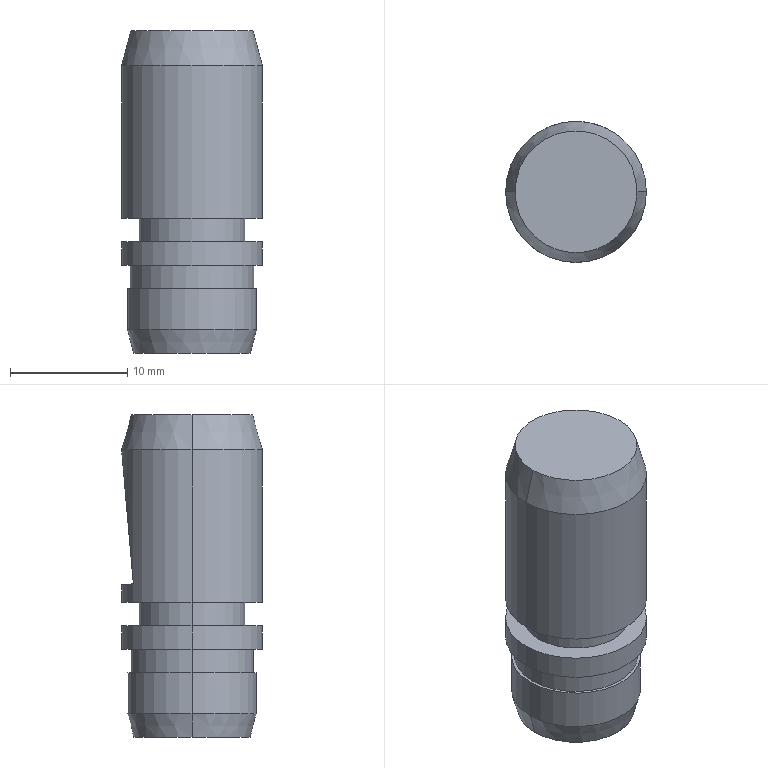Part | STEP file | OP10-113_round-pin | 1 solid | 22 faces | box 12 x 12 x 27.5 mm | volume 2777 mm3 | cylinder 10 | plane 8 | cone 4 | commonest cylinder face diameters 12 x4 9 x2 10.5 x2 11 x2
STEP:
#1=CARTESIAN_POINT('',(0.,0.,0.));
#2=DIRECTION('',(0.,0.,1.));
#3=DIRECTION('',(1.,0.,0.));
#4=AXIS2_PLACEMENT_3D('',#1,#2,#3);
#5=CARTESIAN_POINT('',(4.964,0.,-27.5));
#6=VERTEX_POINT('',#5);
#7=CARTESIAN_POINT('',(-4.964,0.,-27.5));
#8=VERTEX_POINT('',#7);
#9=CARTESIAN_POINT('',(0.,0.,-27.5));
#10=DIRECTION('',(0.,0.,1.));
#11=DIRECTION('',(1.,0.,0.));
#12=AXIS2_PLACEMENT_3D('',#9,#10,#11);
#13=CIRCLE('',#12,4.964);
#14=CARTESIAN_POINT('',(0.,0.,-27.5));
#15=DIRECTION('',(0.,0.,1.));
#16=DIRECTION('',(1.,0.,0.));
#17=AXIS2_PLACEMENT_3D('',#14,#15,#16);
#18=CONICAL_SURFACE('',#17,4.964,0.2618);
#19=CARTESIAN_POINT('',(0.,0.));
#20=DIRECTION('',(1.,0.));
#21=VECTOR('',#20,1.);
#22=LINE('',#19,#21);
#23=(GEOMETRIC_REPRESENTATION_CONTEXT(2)PARAMETRIC_REPRESENTATION_CONTEXT()REPRESENTATION_CONTEXT('',''));
#24=DEFINITIONAL_REPRESENTATION('',(#22),#23);
#25=PCURVE('',#18,#24);
#26=CARTESIAN_POINT('',(0.,4.964,-27.5));
#27=DIRECTION('',(0.,0.,1.));
#28=DIRECTION('',(1.,0.,0.));
#29=AXIS2_PLACEMENT_3D('',#26,#27,#28);
#30=PLANE('',#29);
#31=CARTESIAN_POINT('',(0.,-4.964));
#32=DIRECTION('',(1.,0.));
#33=AXIS2_PLACEMENT_2D('',#31,#32);
#34=CIRCLE('',#33,4.964);
#35=(GEOMETRIC_REPRESENTATION_CONTEXT(2)PARAMETRIC_REPRESENTATION_CONTEXT()REPRESENTATION_CONTEXT('',''));
#36=DEFINITIONAL_REPRESENTATION('',(#34),#35);
#37=PCURVE('',#30,#36);
#38=SURFACE_CURVE('',#13,(#25,#37),.PCURVE_S1.);
#39=EDGE_CURVE('',#6,#8,#38,.T.);
#40=ORIENTED_EDGE('',*,*,#39,.T.);
#41=CARTESIAN_POINT('',(-5.5,0.,-25.5));
#42=VERTEX_POINT('',#41);
#43=CARTESIAN_POINT('',(-4.964,0.,-27.5));
#44=DIRECTION('',(-0.2588,0.,0.9659));
#45=VECTOR('',#44,1.);
#46=LINE('',#43,#45);
#47=CARTESIAN_POINT('',(3.142,0.));
#48=DIRECTION('',(0.,1.));
#49=VECTOR('',#48,1.);
#50=LINE('',#47,#49);
#51=(GEOMETRIC_REPRESENTATION_CONTEXT(2)PARAMETRIC_REPRESENTATION_CONTEXT()REPRESENTATION_CONTEXT('',''));
#52=DEFINITIONAL_REPRESENTATION('',(#50),#51);
#53=PCURVE('',#18,#52);
#54=CARTESIAN_POINT('',(0.,0.,-27.5));
#55=DIRECTION('',(0.,0.,1.));
#56=DIRECTION('',(1.,0.,0.));
#57=AXIS2_PLACEMENT_3D('',#54,#55,#56);
#58=CONICAL_SURFACE('',#57,4.964,0.2618);
#59=CARTESIAN_POINT('',(3.142,0.));
#60=DIRECTION('',(0.,1.));
#61=VECTOR('',#60,1.);
#62=LINE('',#59,#61);
#63=(GEOMETRIC_REPRESENTATION_CONTEXT(2)PARAMETRIC_REPRESENTATION_CONTEXT()REPRESENTATION_CONTEXT('',''));
#64=DEFINITIONAL_REPRESENTATION('',(#62),#63);
#65=PCURVE('',#58,#64);
#66=SURFACE_CURVE('',#46,(#53,#65),.PCURVE_S1.);
#67=EDGE_CURVE('',#8,#42,#66,.T.);
#68=ORIENTED_EDGE('',*,*,#67,.T.);
#69=CARTESIAN_POINT('',(5.5,0.,-25.5));
#70=VERTEX_POINT('',#69);
#71=CARTESIAN_POINT('',(0.,0.,-25.5));
#72=DIRECTION('',(0.,0.,1.));
#73=DIRECTION('',(1.,0.,0.));
#74=AXIS2_PLACEMENT_3D('',#71,#72,#73);
#75=CIRCLE('',#74,5.5);
#76=CARTESIAN_POINT('',(0.,2.));
#77=DIRECTION('',(1.,0.));
#78=VECTOR('',#77,1.);
#79=LINE('',#76,#78);
#80=(GEOMETRIC_REPRESENTATION_CONTEXT(2)PARAMETRIC_REPRESENTATION_CONTEXT()REPRESENTATION_CONTEXT('',''));
#81=DEFINITIONAL_REPRESENTATION('',(#79),#80);
#82=PCURVE('',#18,#81);
#83=CARTESIAN_POINT('',(0.,0.,0.));
#84=DIRECTION('',(0.,0.,1.));
#85=DIRECTION('',(1.,0.,0.));
#86=AXIS2_PLACEMENT_3D('',#83,#84,#85);
#87=CYLINDRICAL_SURFACE('',#86,5.5);
#88=CARTESIAN_POINT('',(0.,-25.5));
#89=DIRECTION('',(1.,0.));
#90=VECTOR('',#89,1.);
#91=LINE('',#88,#90);
#92=(GEOMETRIC_REPRESENTATION_CONTEXT(2)PARAMETRIC_REPRESENTATION_CONTEXT()REPRESENTATION_CONTEXT('',''));
#93=DEFINITIONAL_REPRESENTATION('',(#91),#92);
#94=PCURVE('',#87,#93);
#95=SURFACE_CURVE('',#75,(#82,#94),.PCURVE_S1.);
#96=EDGE_CURVE('',#70,#42,#95,.T.);
#97=ORIENTED_EDGE('',*,*,#96,.F.);
#98=CARTESIAN_POINT('',(4.964,0.,-27.5));
#99=DIRECTION('',(0.2588,0.,0.9659));
#100=VECTOR('',#99,1.);
#101=LINE('',#98,#100);
#102=CARTESIAN_POINT('',(0.,0.));
#103=DIRECTION('',(0.,1.));
#104=VECTOR('',#103,1.);
#105=LINE('',#102,#104);
#106=(GEOMETRIC_REPRESENTATION_CONTEXT(2)PARAMETRIC_REPRESENTATION_CONTEXT()REPRESENTATION_CONTEXT('',''));
#107=DEFINITIONAL_REPRESENTATION('',(#105),#106);
#108=PCURVE('',#18,#107);
#109=CARTESIAN_POINT('',(6.283,0.));
#110=DIRECTION('',(0.,1.));
#111=VECTOR('',#110,1.);
#112=LINE('',#109,#111);
#113=(GEOMETRIC_REPRESENTATION_CONTEXT(2)PARAMETRIC_REPRESENTATION_CONTEXT()REPRESENTATION_CONTEXT('',''));
#114=DEFINITIONAL_REPRESENTATION('',(#112),#113);
#115=PCURVE('',#58,#114);
#116=SURFACE_CURVE('',#101,(#108,#115),.PCURVE_S1.);
#117=EDGE_CURVE('',#6,#70,#116,.T.);
#118=ORIENTED_EDGE('',*,*,#117,.F.);
#119=EDGE_LOOP('',(#40,#68,#97,#118));
#120=FACE_BOUND('',#119,.T.);
#121=ADVANCED_FACE('',(#120),#18,.T.);
#122=ORIENTED_EDGE('',*,*,#96,.T.);
#123=CARTESIAN_POINT('',(-5.5,0.,-22.));
#124=VERTEX_POINT('',#123);
#125=CARTESIAN_POINT('',(-5.5,0.,0.));
#126=DIRECTION('',(0.,0.,1.));
#127=VECTOR('',#126,1.);
#128=LINE('',#125,#127);
#129=CARTESIAN_POINT('',(3.142,0.));
#130=DIRECTION('',(0.,1.));
#131=VECTOR('',#130,1.);
#132=LINE('',#129,#131);
#133=(GEOMETRIC_REPRESENTATION_CONTEXT(2)PARAMETRIC_REPRESENTATION_CONTEXT()REPRESENTATION_CONTEXT('',''));
#134=DEFINITIONAL_REPRESENTATION('',(#132),#133);
#135=PCURVE('',#87,#134);
#136=CARTESIAN_POINT('',(0.,0.,0.));
#137=DIRECTION('',(0.,0.,1.));
#138=DIRECTION('',(1.,0.,0.));
#139=AXIS2_PLACEMENT_3D('',#136,#137,#138);
#140=CYLINDRICAL_SURFACE('',#139,5.5);
#141=CARTESIAN_POINT('',(3.142,0.));
#142=DIRECTION('',(0.,1.));
#143=VECTOR('',#142,1.);
#144=LINE('',#141,#143);
#145=(GEOMETRIC_REPRESENTATION_CONTEXT(2)PARAMETRIC_REPRESENTATION_CONTEXT()REPRESENTATION_CONTEXT('',''));
#146=DEFINITIONAL_REPRESENTATION('',(#144),#145);
#147=PCURVE('',#140,#146);
#148=SURFACE_CURVE('',#128,(#135,#147),.PCURVE_S1.);
#149=EDGE_CURVE('',#42,#124,#148,.T.);
#150=ORIENTED_EDGE('',*,*,#149,.T.);
#151=CARTESIAN_POINT('',(5.5,0.,-22.));
#152=VERTEX_POINT('',#151);
#153=CARTESIAN_POINT('',(0.,0.,-22.));
#154=DIRECTION('',(0.,0.,1.));
#155=DIRECTION('',(1.,0.,0.));
#156=AXIS2_PLACEMENT_3D('',#153,#154,#155);
#157=CIRCLE('',#156,5.5);
#158=CARTESIAN_POINT('',(0.,-22.));
#159=DIRECTION('',(1.,0.));
#160=VECTOR('',#159,1.);
#161=LINE('',#158,#160);
#162=(GEOMETRIC_REPRESENTATION_CONTEXT(2)PARAMETRIC_REPRESENTATION_CONTEXT()REPRESENTATION_CONTEXT('',''));
#163=DEFINITIONAL_REPRESENTATION('',(#161),#162);
#164=PCURVE('',#87,#163);
#165=CARTESIAN_POINT('',(0.,5.25,-22.));
#166=DIRECTION('',(0.,0.,-1.));
#167=DIRECTION('',(-1.,0.,0.));
#168=AXIS2_PLACEMENT_3D('',#165,#166,#167);
#169=PLANE('',#168);
#170=CARTESIAN_POINT('',(-5.5,-5.25));
#171=CARTESIAN_POINT('',(-5.5,4.276));
#172=CARTESIAN_POINT('',(2.75,-0.4869));
#173=CARTESIAN_POINT('',(11.,-5.25));
#174=CARTESIAN_POINT('',(2.75,-10.013));
#175=CARTESIAN_POINT('',(-5.5,-14.776));
#176=CARTESIAN_POINT('',(-5.5,-5.25));
#177=(BOUNDED_CURVE()B_SPLINE_CURVE(2,(#170,#171,#172,#173,#174,#175,#176),.UNSPECIFIED.,.T.,.F.)B_SPLINE_CURVE_WITH_KNOTS((1,2,2,2,2,1),(-2.094,0.,2.094,4.189,6.283,8.378),.UNSPECIFIED.)CURVE()GEOMETRIC_REPRESENTATION_ITEM()RATIONAL_B_SPLINE_CURVE((1.,0.5,1.,0.5,1.,0.5,1.))REPRESENTATION_ITEM(''));
#178=(GEOMETRIC_REPRESENTATION_CONTEXT(2)PARAMETRIC_REPRESENTATION_CONTEXT()REPRESENTATION_CONTEXT('',''));
#179=DEFINITIONAL_REPRESENTATION('',(#177),#178);
#180=PCURVE('',#169,#179);
#181=SURFACE_CURVE('',#157,(#164,#180),.PCURVE_S1.);
#182=EDGE_CURVE('',#152,#124,#181,.T.);
#183=ORIENTED_EDGE('',*,*,#182,.F.);
#184=CARTESIAN_POINT('',(5.5,0.,0.));
#185=DIRECTION('',(0.,0.,1.));
#186=VECTOR('',#185,1.);
#187=LINE('',#184,#186);
#188=CARTESIAN_POINT('',(0.,0.));
#189=DIRECTION('',(0.,1.));
#190=VECTOR('',#189,1.);
#191=LINE('',#188,#190);
#192=(GEOMETRIC_REPRESENTATION_CONTEXT(2)PARAMETRIC_REPRESENTATION_CONTEXT()REPRESENTATION_CONTEXT('',''));
#193=DEFINITIONAL_REPRESENTATION('',(#191),#192);
#194=PCURVE('',#87,#193);
#195=CARTESIAN_POINT('',(6.283,0.));
#196=DIRECTION('',(0.,1.));
#197=VECTOR('',#196,1.);
#198=LINE('',#195,#197);
#199=(GEOMETRIC_REPRESENTATION_CONTEXT(2)PARAMETRIC_REPRESENTATION_CONTEXT()REPRESENTATION_CONTEXT('',''));
#200=DEFINITIONAL_REPRESENTATION('',(#198),#199);
#201=PCURVE('',#140,#200);
#202=SURFACE_CURVE('',#187,(#194,#201),.PCURVE_S1.);
#203=EDGE_CURVE('',#70,#152,#202,.T.);
#204=ORIENTED_EDGE('',*,*,#203,.F.);
#205=EDGE_LOOP('',(#122,#150,#183,#204));
#206=FACE_BOUND('',#205,.T.);
#207=ADVANCED_FACE('',(#206),#87,.T.);
#208=CARTESIAN_POINT('',(5.25,0.,-22.));
#209=VERTEX_POINT('',#208);
#210=CARTESIAN_POINT('',(-5.25,0.,-22.));
#211=VERTEX_POINT('',#210);
#212=CARTESIAN_POINT('',(0.,0.,-22.));
#213=DIRECTION('',(0.,0.,1.));
#214=DIRECTION('',(1.,0.,0.));
#215=AXIS2_PLACEMENT_3D('',#212,#213,#214);
#216=CIRCLE('',#215,5.25);
#217=CARTESIAN_POINT('',(0.,0.,0.));
#218=DIRECTION('',(0.,0.,1.));
#219=DIRECTION('',(1.,0.,0.));
#220=AXIS2_PLACEMENT_3D('',#217,#218,#219);
#221=CYLINDRICAL_SURFACE('',#220,5.25);
#222=CARTESIAN_POINT('',(0.,-22.));
#223=DIRECTION('',(1.,0.));
#224=VECTOR('',#223,1.);
#225=LINE('',#222,#224);
#226=(GEOMETRIC_REPRESENTATION_CONTEXT(2)PARAMETRIC_REPRESENTATION_CONTEXT()REPRESENTATION_CONTEXT('',''));
#227=DEFINITIONAL_REPRESENTATION('',(#225),#226);
#228=PCURVE('',#221,#227);
#229=CARTESIAN_POINT('',(-5.25,-5.25));
#230=CARTESIAN_POINT('',(-5.25,3.843));
#231=CARTESIAN_POINT('',(2.625,-0.7034));
#232=CARTESIAN_POINT('',(10.5,-5.25));
#233=CARTESIAN_POINT('',(2.625,-9.797));
#234=CARTESIAN_POINT('',(-5.25,-14.343));
#235=CARTESIAN_POINT('',(-5.25,-5.25));
#236=(BOUNDED_CURVE()B_SPLINE_CURVE(2,(#229,#230,#231,#232,#233,#234,#235),.UNSPECIFIED.,.T.,.F.)B_SPLINE_CURVE_WITH_KNOTS((1,2,2,2,2,1),(-2.094,0.,2.094,4.189,6.283,8.378),.UNSPECIFIED.)CURVE()GEOMETRIC_REPRESENTATION_ITEM()RATIONAL_B_SPLINE_CURVE((1.,0.5,1.,0.5,1.,0.5,1.))REPRESENTATION_ITEM(''));
#237=(GEOMETRIC_REPRESENTATION_CONTEXT(2)PARAMETRIC_REPRESENTATION_CONTEXT()REPRESENTATION_CONTEXT('',''));
#238=DEFINITIONAL_REPRESENTATION('',(#236),#237);
#239=PCURVE('',#169,#238);
#240=SURFACE_CURVE('',#216,(#228,#239),.PCURVE_S1.);
#241=EDGE_CURVE('',#209,#211,#240,.T.);
#242=ORIENTED_EDGE('',*,*,#241,.T.);
#243=CARTESIAN_POINT('',(-5.25,0.,-20.));
#244=VERTEX_POINT('',#243);
#245=CARTESIAN_POINT('',(-5.25,0.,0.));
#246=DIRECTION('',(0.,0.,1.));
#247=VECTOR('',#246,1.);
#248=LINE('',#245,#247);
#249=CARTESIAN_POINT('',(3.142,0.));
#250=DIRECTION('',(0.,1.));
#251=VECTOR('',#250,1.);
#252=LINE('',#249,#251);
#253=(GEOMETRIC_REPRESENTATION_CONTEXT(2)PARAMETRIC_REPRESENTATION_CONTEXT()REPRESENTATION_CONTEXT('',''));
#254=DEFINITIONAL_REPRESENTATION('',(#252),#253);
#255=PCURVE('',#221,#254);
#256=CARTESIAN_POINT('',(0.,0.,0.));
#257=DIRECTION('',(0.,0.,1.));
#258=DIRECTION('',(1.,0.,0.));
#259=AXIS2_PLACEMENT_3D('',#256,#257,#258);
#260=CYLINDRICAL_SURFACE('',#259,5.25);
#261=CARTESIAN_POINT('',(3.142,0.));
#262=DIRECTION('',(0.,1.));
#263=VECTOR('',#262,1.);
#264=LINE('',#261,#263);
#265=(GEOMETRIC_REPRESENTATION_CONTEXT(2)PARAMETRIC_REPRESENTATION_CONTEXT()REPRESENTATION_CONTEXT('',''));
#266=DEFINITIONAL_REPRESENTATION('',(#264),#265);
#267=PCURVE('',#260,#266);
#268=SURFACE_CURVE('',#248,(#255,#267),.PCURVE_S1.);
#269=EDGE_CURVE('',#211,#244,#268,.T.);
#270=ORIENTED_EDGE('',*,*,#269,.T.);
#271=CARTESIAN_POINT('',(5.25,0.,-20.));
#272=VERTEX_POINT('',#271);
#273=CARTESIAN_POINT('',(0.,0.,-20.));
#274=DIRECTION('',(0.,0.,1.));
#275=DIRECTION('',(1.,0.,0.));
#276=AXIS2_PLACEMENT_3D('',#273,#274,#275);
#277=CIRCLE('',#276,5.25);
#278=CARTESIAN_POINT('',(0.,-20.));
#279=DIRECTION('',(1.,0.));
#280=VECTOR('',#279,1.);
#281=LINE('',#278,#280);
#282=(GEOMETRIC_REPRESENTATION_CONTEXT(2)PARAMETRIC_REPRESENTATION_CONTEXT()REPRESENTATION_CONTEXT('',''));
#283=DEFINITIONAL_REPRESENTATION('',(#281),#282);
#284=PCURVE('',#221,#283);
#285=CARTESIAN_POINT('',(0.,5.25,-20.));
#286=DIRECTION('',(0.,0.,1.));
#287=DIRECTION('',(1.,0.,0.));
#288=AXIS2_PLACEMENT_3D('',#285,#286,#287);
#289=PLANE('',#288);
#290=CARTESIAN_POINT('',(0.,-5.25));
#291=DIRECTION('',(1.,0.));
#292=AXIS2_PLACEMENT_2D('',#290,#291);
#293=CIRCLE('',#292,5.25);
#294=(GEOMETRIC_REPRESENTATION_CONTEXT(2)PARAMETRIC_REPRESENTATION_CONTEXT()REPRESENTATION_CONTEXT('',''));
#295=DEFINITIONAL_REPRESENTATION('',(#293),#294);
#296=PCURVE('',#289,#295);
#297=SURFACE_CURVE('',#277,(#284,#296),.PCURVE_S1.);
#298=EDGE_CURVE('',#272,#244,#297,.T.);
#299=ORIENTED_EDGE('',*,*,#298,.F.);
#300=CARTESIAN_POINT('',(5.25,0.,0.));
#301=DIRECTION('',(0.,0.,1.));
#302=VECTOR('',#301,1.);
#303=LINE('',#300,#302);
#304=CARTESIAN_POINT('',(0.,0.));
#305=DIRECTION('',(0.,1.));
#306=VECTOR('',#305,1.);
#307=LINE('',#304,#306);
#308=(GEOMETRIC_REPRESENTATION_CONTEXT(2)PARAMETRIC_REPRESENTATION_CONTEXT()REPRESENTATION_CONTEXT('',''));
#309=DEFINITIONAL_REPRESENTATION('',(#307),#308);
#310=PCURVE('',#221,#309);
#311=CARTESIAN_POINT('',(6.283,0.));
#312=DIRECTION('',(0.,1.));
#313=VECTOR('',#312,1.);
#314=LINE('',#311,#313);
#315=(GEOMETRIC_REPRESENTATION_CONTEXT(2)PARAMETRIC_REPRESENTATION_CONTEXT()REPRESENTATION_CONTEXT('',''));
#316=DEFINITIONAL_REPRESENTATION('',(#314),#315);
#317=PCURVE('',#260,#316);
#318=SURFACE_CURVE('',#303,(#310,#317),.PCURVE_S1.);
#319=EDGE_CURVE('',#209,#272,#318,.T.);
#320=ORIENTED_EDGE('',*,*,#319,.F.);
#321=EDGE_LOOP('',(#242,#270,#299,#320));
#322=FACE_BOUND('',#321,.T.);
#323=ADVANCED_FACE('',(#322),#221,.T.);
#324=CARTESIAN_POINT('',(6.,0.,-20.));
#325=VERTEX_POINT('',#324);
#326=CARTESIAN_POINT('',(-6.,0.,-20.));
#327=VERTEX_POINT('',#326);
#328=CARTESIAN_POINT('',(0.,0.,-20.));
#329=DIRECTION('',(0.,0.,1.));
#330=DIRECTION('',(1.,0.,0.));
#331=AXIS2_PLACEMENT_3D('',#328,#329,#330);
#332=CIRCLE('',#331,6.);
#333=CARTESIAN_POINT('',(0.,0.,0.));
#334=DIRECTION('',(0.,0.,1.));
#335=DIRECTION('',(1.,0.,0.));
#336=AXIS2_PLACEMENT_3D('',#333,#334,#335);
#337=CYLINDRICAL_SURFACE('',#336,6.);
#338=CARTESIAN_POINT('',(0.,-20.));
#339=DIRECTION('',(1.,0.));
#340=VECTOR('',#339,1.);
#341=LINE('',#338,#340);
#342=(GEOMETRIC_REPRESENTATION_CONTEXT(2)PARAMETRIC_REPRESENTATION_CONTEXT()REPRESENTATION_CONTEXT('',''));
#343=DEFINITIONAL_REPRESENTATION('',(#341),#342);
#344=PCURVE('',#337,#343);
#345=CARTESIAN_POINT('',(0.,-5.25));
#346=DIRECTION('',(1.,0.));
#347=AXIS2_PLACEMENT_2D('',#345,#346);
#348=CIRCLE('',#347,6.);
#349=(GEOMETRIC_REPRESENTATION_CONTEXT(2)PARAMETRIC_REPRESENTATION_CONTEXT()REPRESENTATION_CONTEXT('',''));
#350=DEFINITIONAL_REPRESENTATION('',(#348),#349);
#351=PCURVE('',#289,#350);
#352=SURFACE_CURVE('',#332,(#344,#351),.PCURVE_S1.);
#353=EDGE_CURVE('',#325,#327,#352,.T.);
#354=ORIENTED_EDGE('',*,*,#353,.T.);
#355=CARTESIAN_POINT('',(-6.,0.,-18.));
#356=VERTEX_POINT('',#355);
#357=CARTESIAN_POINT('',(-6.,0.,0.));
#358=DIRECTION('',(0.,0.,1.));
#359=VECTOR('',#358,1.);
#360=LINE('',#357,#359);
#361=CARTESIAN_POINT('',(3.142,0.));
#362=DIRECTION('',(0.,1.));
#363=VECTOR('',#362,1.);
#364=LINE('',#361,#363);
#365=(GEOMETRIC_REPRESENTATION_CONTEXT(2)PARAMETRIC_REPRESENTATION_CONTEXT()REPRESENTATION_CONTEXT('',''));
#366=DEFINITIONAL_REPRESENTATION('',(#364),#365);
#367=PCURVE('',#337,#366);
#368=CARTESIAN_POINT('',(0.,0.,0.));
#369=DIRECTION('',(0.,0.,1.));
#370=DIRECTION('',(1.,0.,0.));
#371=AXIS2_PLACEMENT_3D('',#368,#369,#370);
#372=CYLINDRICAL_SURFACE('',#371,6.);
#373=CARTESIAN_POINT('',(3.142,0.));
#374=DIRECTION('',(0.,1.));
#375=VECTOR('',#374,1.);
#376=LINE('',#373,#375);
#377=(GEOMETRIC_REPRESENTATION_CONTEXT(2)PARAMETRIC_REPRESENTATION_CONTEXT()REPRESENTATION_CONTEXT('',''));
#378=DEFINITIONAL_REPRESENTATION('',(#376),#377);
#379=PCURVE('',#372,#378);
#380=SURFACE_CURVE('',#360,(#367,#379),.PCURVE_S1.);
#381=EDGE_CURVE('',#327,#356,#380,.T.);
#382=ORIENTED_EDGE('',*,*,#381,.T.);
#383=CARTESIAN_POINT('',(6.,0.,-18.));
#384=VERTEX_POINT('',#383);
#385=CARTESIAN_POINT('',(0.,0.,-18.));
#386=DIRECTION('',(0.,0.,1.));
#387=DIRECTION('',(1.,0.,0.));
#388=AXIS2_PLACEMENT_3D('',#385,#386,#387);
#389=CIRCLE('',#388,6.);
#390=CARTESIAN_POINT('',(0.,-18.));
#391=DIRECTION('',(1.,0.));
#392=VECTOR('',#391,1.);
#393=LINE('',#390,#392);
#394=(GEOMETRIC_REPRESENTATION_CONTEXT(2)PARAMETRIC_REPRESENTATION_CONTEXT()REPRESENTATION_CONTEXT('',''));
#395=DEFINITIONAL_REPRESENTATION('',(#393),#394);
#396=PCURVE('',#337,#395);
#397=CARTESIAN_POINT('',(0.,4.5,-18.));
#398=DIRECTION('',(0.,0.,-1.));
#399=DIRECTION('',(-1.,0.,0.));
#400=AXIS2_PLACEMENT_3D('',#397,#398,#399);
#401=PLANE('',#400);
#402=CARTESIAN_POINT('',(-6.,-4.5));
#403=CARTESIAN_POINT('',(-6.,5.892));
#404=CARTESIAN_POINT('',(3.,0.6962));
#405=CARTESIAN_POINT('',(12.,-4.5));
#406=CARTESIAN_POINT('',(3.,-9.696));
#407=CARTESIAN_POINT('',(-6.,-14.892));
#408=CARTESIAN_POINT('',(-6.,-4.5));
#409=(BOUNDED_CURVE()B_SPLINE_CURVE(2,(#402,#403,#404,#405,#406,#407,#408),.UNSPECIFIED.,.T.,.F.)B_SPLINE_CURVE_WITH_KNOTS((1,2,2,2,2,1),(-2.094,0.,2.094,4.189,6.283,8.378),.UNSPECIFIED.)CURVE()GEOMETRIC_REPRESENTATION_ITEM()RATIONAL_B_SPLINE_CURVE((1.,0.5,1.,0.5,1.,0.5,1.))REPRESENTATION_ITEM(''));
#410=(GEOMETRIC_REPRESENTATION_CONTEXT(2)PARAMETRIC_REPRESENTATION_CONTEXT()REPRESENTATION_CONTEXT('',''));
#411=DEFINITIONAL_REPRESENTATION('',(#409),#410);
#412=PCURVE('',#401,#411);
#413=SURFACE_CURVE('',#389,(#396,#412),.PCURVE_S1.);
#414=EDGE_CURVE('',#384,#356,#413,.T.);
#415=ORIENTED_EDGE('',*,*,#414,.F.);
#416=CARTESIAN_POINT('',(6.,0.,0.));
#417=DIRECTION('',(0.,0.,1.));
#418=VECTOR('',#417,1.);
#419=LINE('',#416,#418);
#420=CARTESIAN_POINT('',(0.,0.));
#421=DIRECTION('',(0.,1.));
#422=VECTOR('',#421,1.);
#423=LINE('',#420,#422);
#424=(GEOMETRIC_REPRESENTATION_CONTEXT(2)PARAMETRIC_REPRESENTATION_CONTEXT()REPRESENTATION_CONTEXT('',''));
#425=DEFINITIONAL_REPRESENTATION('',(#423),#424);
#426=PCURVE('',#337,#425);
#427=CARTESIAN_POINT('',(6.283,0.));
#428=DIRECTION('',(0.,1.));
#429=VECTOR('',#428,1.);
#430=LINE('',#427,#429);
#431=(GEOMETRIC_REPRESENTATION_CONTEXT(2)PARAMETRIC_REPRESENTATION_CONTEXT()REPRESENTATION_CONTEXT('',''));
#432=DEFINITIONAL_REPRESENTATION('',(#430),#431);
#433=PCURVE('',#372,#432);
#434=SURFACE_CURVE('',#419,(#426,#433),.PCURVE_S1.);
#435=EDGE_CURVE('',#325,#384,#434,.T.);
#436=ORIENTED_EDGE('',*,*,#435,.F.);
#437=EDGE_LOOP('',(#354,#382,#415,#436));
#438=FACE_BOUND('',#437,.T.);
#439=ADVANCED_FACE('',(#438),#337,.T.);
#440=CARTESIAN_POINT('',(4.5,0.,-18.));
#441=VERTEX_POINT('',#440);
#442=CARTESIAN_POINT('',(-4.5,0.,-18.));
#443=VERTEX_POINT('',#442);
#444=CARTESIAN_POINT('',(0.,0.,-18.));
#445=DIRECTION('',(0.,0.,1.));
#446=DIRECTION('',(1.,0.,0.));
#447=AXIS2_PLACEMENT_3D('',#444,#445,#446);
#448=CIRCLE('',#447,4.5);
#449=CARTESIAN_POINT('',(0.,0.,0.));
#450=DIRECTION('',(0.,0.,1.));
#451=DIRECTION('',(1.,0.,0.));
#452=AXIS2_PLACEMENT_3D('',#449,#450,#451);
#453=CYLINDRICAL_SURFACE('',#452,4.5);
#454=CARTESIAN_POINT('',(0.,-18.));
#455=DIRECTION('',(1.,0.));
#456=VECTOR('',#455,1.);
#457=LINE('',#454,#456);
#458=(GEOMETRIC_REPRESENTATION_CONTEXT(2)PARAMETRIC_REPRESENTATION_CONTEXT()REPRESENTATION_CONTEXT('',''));
#459=DEFINITIONAL_REPRESENTATION('',(#457),#458);
#460=PCURVE('',#453,#459);
#461=CARTESIAN_POINT('',(-4.5,-4.5));
#462=CARTESIAN_POINT('',(-4.5,3.294));
#463=CARTESIAN_POINT('',(2.25,-0.6029));
#464=CARTESIAN_POINT('',(9.,-4.5));
#465=CARTESIAN_POINT('',(2.25,-8.397));
#466=CARTESIAN_POINT('',(-4.5,-12.294));
#467=CARTESIAN_POINT('',(-4.5,-4.5));
#468=(BOUNDED_CURVE()B_SPLINE_CURVE(2,(#461,#462,#463,#464,#465,#466,#467),.UNSPECIFIED.,.T.,.F.)B_SPLINE_CURVE_WITH_KNOTS((1,2,2,2,2,1),(-2.094,0.,2.094,4.189,6.283,8.378),.UNSPECIFIED.)CURVE()GEOMETRIC_REPRESENTATION_ITEM()RATIONAL_B_SPLINE_CURVE((1.,0.5,1.,0.5,1.,0.5,1.))REPRESENTATION_ITEM(''));
#469=(GEOMETRIC_REPRESENTATION_CONTEXT(2)PARAMETRIC_REPRESENTATION_CONTEXT()REPRESENTATION_CONTEXT('',''));
#470=DEFINITIONAL_REPRESENTATION('',(#468),#469);
#471=PCURVE('',#401,#470);
#472=SURFACE_CURVE('',#448,(#460,#471),.PCURVE_S1.);
#473=EDGE_CURVE('',#441,#443,#472,.T.);
#474=ORIENTED_EDGE('',*,*,#473,.T.);
#475=CARTESIAN_POINT('',(-4.5,0.,-16.));
#476=VERTEX_POINT('',#475);
#477=CARTESIAN_POINT('',(-4.5,0.,0.));
#478=DIRECTION('',(0.,0.,1.));
#479=VECTOR('',#478,1.);
#480=LINE('',#477,#479);
#481=CARTESIAN_POINT('',(3.142,0.));
#482=DIRECTION('',(0.,1.));
#483=VECTOR('',#482,1.);
#484=LINE('',#481,#483);
#485=(GEOMETRIC_REPRESENTATION_CONTEXT(2)PARAMETRIC_REPRESENTATION_CONTEXT()REPRESENTATION_CONTEXT('',''));
#486=DEFINITIONAL_REPRESENTATION('',(#484),#485);
#487=PCURVE('',#453,#486);
#488=CARTESIAN_POINT('',(0.,0.,0.));
#489=DIRECTION('',(0.,0.,1.));
#490=DIRECTION('',(1.,0.,0.));
#491=AXIS2_PLACEMENT_3D('',#488,#489,#490);
#492=CYLINDRICAL_SURFACE('',#491,4.5);
#493=CARTESIAN_POINT('',(3.142,0.));
#494=DIRECTION('',(0.,1.));
#495=VECTOR('',#494,1.);
#496=LINE('',#493,#495);
#497=(GEOMETRIC_REPRESENTATION_CONTEXT(2)PARAMETRIC_REPRESENTATION_CONTEXT()REPRESENTATION_CONTEXT('',''));
#498=DEFINITIONAL_REPRESENTATION('',(#496),#497);
#499=PCURVE('',#492,#498);
#500=SURFACE_CURVE('',#480,(#487,#499),.PCURVE_S1.);
#501=EDGE_CURVE('',#443,#476,#500,.T.);
#502=ORIENTED_EDGE('',*,*,#501,.T.);
#503=CARTESIAN_POINT('',(4.5,0.,-16.));
#504=VERTEX_POINT('',#503);
#505=CARTESIAN_POINT('',(0.,0.,-16.));
#506=DIRECTION('',(0.,0.,1.));
#507=DIRECTION('',(1.,0.,0.));
#508=AXIS2_PLACEMENT_3D('',#505,#506,#507);
#509=CIRCLE('',#508,4.5);
#510=CARTESIAN_POINT('',(0.,-16.));
#511=DIRECTION('',(1.,0.));
#512=VECTOR('',#511,1.);
#513=LINE('',#510,#512);
#514=(GEOMETRIC_REPRESENTATION_CONTEXT(2)PARAMETRIC_REPRESENTATION_CONTEXT()REPRESENTATION_CONTEXT('',''));
#515=DEFINITIONAL_REPRESENTATION('',(#513),#514);
#516=PCURVE('',#453,#515);
#517=CARTESIAN_POINT('',(0.,6.,-16.));
#518=DIRECTION('',(0.,0.,1.));
#519=DIRECTION('',(1.,0.,0.));
#520=AXIS2_PLACEMENT_3D('',#517,#518,#519);
#521=PLANE('',#520);
#522=CARTESIAN_POINT('',(0.,-6.));
#523=DIRECTION('',(1.,0.));
#524=AXIS2_PLACEMENT_2D('',#522,#523);
#525=CIRCLE('',#524,4.5);
#526=(GEOMETRIC_REPRESENTATION_CONTEXT(2)PARAMETRIC_REPRESENTATION_CONTEXT()REPRESENTATION_CONTEXT('',''));
#527=DEFINITIONAL_REPRESENTATION('',(#525),#526);
#528=PCURVE('',#521,#527);
#529=SURFACE_CURVE('',#509,(#516,#528),.PCURVE_S1.);
#530=EDGE_CURVE('',#504,#476,#529,.T.);
#531=ORIENTED_EDGE('',*,*,#530,.F.);
#532=CARTESIAN_POINT('',(4.5,0.,0.));
#533=DIRECTION('',(0.,0.,1.));
#534=VECTOR('',#533,1.);
#535=LINE('',#532,#534);
#536=CARTESIAN_POINT('',(0.,0.));
#537=DIRECTION('',(0.,1.));
#538=VECTOR('',#537,1.);
#539=LINE('',#536,#538);
#540=(GEOMETRIC_REPRESENTATION_CONTEXT(2)PARAMETRIC_REPRESENTATION_CONTEXT()REPRESENTATION_CONTEXT('',''));
#541=DEFINITIONAL_REPRESENTATION('',(#539),#540);
#542=PCURVE('',#453,#541);
#543=CARTESIAN_POINT('',(6.283,0.));
#544=DIRECTION('',(0.,1.));
#545=VECTOR('',#544,1.);
#546=LINE('',#543,#545);
#547=(GEOMETRIC_REPRESENTATION_CONTEXT(2)PARAMETRIC_REPRESENTATION_CONTEXT()REPRESENTATION_CONTEXT('',''));
#548=DEFINITIONAL_REPRESENTATION('',(#546),#547);
#549=PCURVE('',#492,#548);
#550=SURFACE_CURVE('',#535,(#542,#549),.PCURVE_S1.);
#551=EDGE_CURVE('',#441,#504,#550,.T.);
#552=ORIENTED_EDGE('',*,*,#551,.F.);
#553=EDGE_LOOP('',(#474,#502,#531,#552));
#554=FACE_BOUND('',#553,.T.);
#555=ADVANCED_FACE('',(#554),#453,.T.);
#556=CARTESIAN_POINT('',(3.311,5.004,-14.413));
#557=VERTEX_POINT('',#556);
#558=CARTESIAN_POINT('',(-3.311,5.004,-14.413));
#559=VERTEX_POINT('',#558);
#560=CARTESIAN_POINT('',(3.311,5.004,-14.413));
#561=CARTESIAN_POINT('',(1.241,6.373,1.242));
#562=CARTESIAN_POINT('',(-1.241,6.373,1.242));
#563=CARTESIAN_POINT('',(-3.311,5.004,-14.413));
#564=(BOUNDED_CURVE()B_SPLINE_CURVE(3,(#560,#561,#562,#563),.UNSPECIFIED.,.F.,.F.)B_SPLINE_CURVE_WITH_KNOTS((4,4),(5.699,6.868),.PIECEWISE_BEZIER_KNOTS.)CURVE()GEOMETRIC_REPRESENTATION_ITEM()RATIONAL_B_SPLINE_CURVE((1.,0.8893,0.8893,1.))REPRESENTATION_ITEM(''));
#565=CARTESIAN_POINT('',(0.,0.,0.));
#566=DIRECTION('',(0.,0.,1.));
#567=DIRECTION('',(1.,0.,0.));
#568=AXIS2_PLACEMENT_3D('',#565,#566,#567);
#569=CYLINDRICAL_SURFACE('',#568,6.);
#570=CARTESIAN_POINT('',(0.9863,-14.413));
#571=CARTESIAN_POINT('',(1.003,-13.78));
#572=CARTESIAN_POINT('',(1.037,-12.553));
#573=CARTESIAN_POINT('',(1.088,-10.84));
#574=CARTESIAN_POINT('',(1.14,-9.269));
#575=CARTESIAN_POINT('',(1.192,-7.85));
#576=CARTESIAN_POINT('',(1.245,-6.595));
#577=CARTESIAN_POINT('',(1.299,-5.514));
#578=CARTESIAN_POINT('',(1.353,-4.617));
#579=CARTESIAN_POINT('',(1.407,-3.911));
#580=CARTESIAN_POINT('',(1.461,-3.402));
#581=CARTESIAN_POINT('',(1.516,-3.095));
#582=CARTESIAN_POINT('',(1.571,-2.992));
#583=CARTESIAN_POINT('',(1.626,-3.095));
#584=CARTESIAN_POINT('',(1.68,-3.402));
#585=CARTESIAN_POINT('',(1.735,-3.911));
#586=CARTESIAN_POINT('',(1.789,-4.617));
#587=CARTESIAN_POINT('',(1.843,-5.514));
#588=CARTESIAN_POINT('',(1.896,-6.595));
#589=CARTESIAN_POINT('',(1.949,-7.85));
#590=CARTESIAN_POINT('',(2.002,-9.269));
#591=CARTESIAN_POINT('',(2.054,-10.84));
#592=CARTESIAN_POINT('',(2.105,-12.553));
#593=CARTESIAN_POINT('',(2.139,-13.78));
#594=CARTESIAN_POINT('',(2.155,-14.413));
#595=B_SPLINE_CURVE_WITH_KNOTS('',3,(#570,#571,#572,#573,#574,#575,#576,#577,#578,#579,#580,#581,#582,#583,#584,#585,#586,#587,#588,#589,#590,#591,#592,#593,#594),.UNSPECIFIED.,.F.,.F.,(4,1,1,1,1,1,1,1,1,1,1,1,1,1,1,1,1,1,1,1,1,1,4),(5.699,5.752,5.805,5.858,5.911,5.964,6.017,6.071,6.124,6.177,6.23,6.283,6.336,6.389,6.443,6.496,6.549,6.602,6.655,6.708,6.761,6.815,6.868),.QUASI_UNIFORM_KNOTS.);
#596=(GEOMETRIC_REPRESENTATION_CONTEXT(2)PARAMETRIC_REPRESENTATION_CONTEXT()REPRESENTATION_CONTEXT('',''));
#597=DEFINITIONAL_REPRESENTATION('',(#595),#596);
#598=PCURVE('',#569,#597);
#599=CARTESIAN_POINT('',(-20.,7.054,9.018));
#600=DIRECTION('',(0.,-0.9962,0.08716));
#601=DIRECTION('',(0.,-0.08716,-0.9962));
#602=AXIS2_PLACEMENT_3D('',#599,#600,#601);
#603=PLANE('',#602);
#604=CARTESIAN_POINT('',(23.52,23.311));
#605=CARTESIAN_POINT('',(7.806,21.241));
#606=CARTESIAN_POINT('',(7.806,18.759));
#607=CARTESIAN_POINT('',(23.52,16.689));
#608=(BOUNDED_CURVE()B_SPLINE_CURVE(3,(#604,#605,#606,#607),.UNSPECIFIED.,.F.,.F.)B_SPLINE_CURVE_WITH_KNOTS((4,4),(5.699,6.868),.PIECEWISE_BEZIER_KNOTS.)CURVE()GEOMETRIC_REPRESENTATION_ITEM()RATIONAL_B_SPLINE_CURVE((1.,0.8893,0.8893,1.))REPRESENTATION_ITEM(''));
#609=(GEOMETRIC_REPRESENTATION_CONTEXT(2)PARAMETRIC_REPRESENTATION_CONTEXT()REPRESENTATION_CONTEXT('',''));
#610=DEFINITIONAL_REPRESENTATION('',(#608),#609);
#611=PCURVE('',#603,#610);
#612=SURFACE_CURVE('',#564,(#598,#611),.PCURVE_S1.);
#613=EDGE_CURVE('',#557,#559,#612,.T.);
#614=ORIENTED_EDGE('',*,*,#613,.T.);
#615=CARTESIAN_POINT('',(-3.311,5.004,-14.413));
#616=CARTESIAN_POINT('',(-1.241,6.373,-14.533));
#617=CARTESIAN_POINT('',(1.241,6.373,-14.533));
#618=CARTESIAN_POINT('',(3.311,5.004,-14.413));
#619=(BOUNDED_CURVE()B_SPLINE_CURVE(3,(#615,#616,#617,#618),.UNSPECIFIED.,.F.,.F.)B_SPLINE_CURVE_WITH_KNOTS((4,4),(2.557,3.726),.PIECEWISE_BEZIER_KNOTS.)CURVE()GEOMETRIC_REPRESENTATION_ITEM()RATIONAL_B_SPLINE_CURVE((1.,0.8893,0.8893,1.))REPRESENTATION_ITEM(''));
#620=CARTESIAN_POINT('',(2.155,-14.413));
#621=CARTESIAN_POINT('',(2.139,-14.418));
#622=CARTESIAN_POINT('',(2.105,-14.427));
#623=CARTESIAN_POINT('',(2.054,-14.44));
#624=CARTESIAN_POINT('',(2.002,-14.452));
#625=CARTESIAN_POINT('',(1.949,-14.463));
#626=CARTESIAN_POINT('',(1.896,-14.473));
#627=CARTESIAN_POINT('',(1.843,-14.481));
#628=CARTESIAN_POINT('',(1.789,-14.488));
#629=CARTESIAN_POINT('',(1.735,-14.493));
#630=CARTESIAN_POINT('',(1.68,-14.497));
#631=CARTESIAN_POINT('',(1.626,-14.499));
#632=CARTESIAN_POINT('',(1.571,-14.5));
#633=CARTESIAN_POINT('',(1.516,-14.499));
#634=CARTESIAN_POINT('',(1.461,-14.497));
#635=CARTESIAN_POINT('',(1.407,-14.493));
#636=CARTESIAN_POINT('',(1.353,-14.488));
#637=CARTESIAN_POINT('',(1.299,-14.481));
#638=CARTESIAN_POINT('',(1.245,-14.473));
#639=CARTESIAN_POINT('',(1.192,-14.463));
#640=CARTESIAN_POINT('',(1.14,-14.452));
#641=CARTESIAN_POINT('',(1.088,-14.44));
#642=CARTESIAN_POINT('',(1.037,-14.427));
#643=CARTESIAN_POINT('',(1.003,-14.418));
#644=CARTESIAN_POINT('',(0.9863,-14.413));
#645=B_SPLINE_CURVE_WITH_KNOTS('',3,(#620,#621,#622,#623,#624,#625,#626,#627,#628,#629,#630,#631,#632,#633,#634,#635,#636,#637,#638,#639,#640,#641,#642,#643,#644),.UNSPECIFIED.,.F.,.F.,(4,1,1,1,1,1,1,1,1,1,1,1,1,1,1,1,1,1,1,1,1,1,4),(2.557,2.61,2.663,2.716,2.77,2.823,2.876,2.929,2.982,3.035,3.088,3.142,3.195,3.248,3.301,3.354,3.407,3.46,3.514,3.567,3.62,3.673,3.726),.QUASI_UNIFORM_KNOTS.);
#646=(GEOMETRIC_REPRESENTATION_CONTEXT(2)PARAMETRIC_REPRESENTATION_CONTEXT()REPRESENTATION_CONTEXT('',''));
#647=DEFINITIONAL_REPRESENTATION('',(#645),#646);
#648=PCURVE('',#569,#647);
#649=CARTESIAN_POINT('',(-20.,6.,-14.5));
#650=DIRECTION('',(0.,-0.08716,-0.9962));
#651=DIRECTION('',(0.,0.9962,-0.08716));
#652=AXIS2_PLACEMENT_3D('',#649,#650,#651);
#653=PLANE('',#652);
#654=CARTESIAN_POINT('',(-1.,16.689));
#655=CARTESIAN_POINT('',(0.3748,18.759));
#656=CARTESIAN_POINT('',(0.3748,21.241));
#657=CARTESIAN_POINT('',(-1.,23.311));
#658=(BOUNDED_CURVE()B_SPLINE_CURVE(3,(#654,#655,#656,#657),.UNSPECIFIED.,.F.,.F.)B_SPLINE_CURVE_WITH_KNOTS((4,4),(2.557,3.726),.PIECEWISE_BEZIER_KNOTS.)CURVE()GEOMETRIC_REPRESENTATION_ITEM()RATIONAL_B_SPLINE_CURVE((1.,0.8893,0.8893,1.))REPRESENTATION_ITEM(''));
#659=(GEOMETRIC_REPRESENTATION_CONTEXT(2)PARAMETRIC_REPRESENTATION_CONTEXT()REPRESENTATION_CONTEXT('',''));
#660=DEFINITIONAL_REPRESENTATION('',(#658),#659);
#661=PCURVE('',#653,#660);
#662=SURFACE_CURVE('',#619,(#648,#661),.PCURVE_S1.);
#663=EDGE_CURVE('',#559,#557,#662,.T.);
#664=ORIENTED_EDGE('',*,*,#663,.T.);
#665=EDGE_LOOP('',(#614,#664));
#666=FACE_BOUND('',#665,.T.);
#667=CARTESIAN_POINT('',(6.,0.,-16.));
#668=VERTEX_POINT('',#667);
#669=CARTESIAN_POINT('',(-6.,0.,-16.));
#670=VERTEX_POINT('',#669);
#671=CARTESIAN_POINT('',(0.,0.,-16.));
#672=DIRECTION('',(0.,0.,1.));
#673=DIRECTION('',(1.,0.,0.));
#674=AXIS2_PLACEMENT_3D('',#671,#672,#673);
#675=CIRCLE('',#674,6.);
#676=CARTESIAN_POINT('',(0.,-16.));
#677=DIRECTION('',(1.,0.));
#678=VECTOR('',#677,1.);
#679=LINE('',#676,#678);
#680=(GEOMETRIC_REPRESENTATION_CONTEXT(2)PARAMETRIC_REPRESENTATION_CONTEXT()REPRESENTATION_CONTEXT('',''));
#681=DEFINITIONAL_REPRESENTATION('',(#679),#680);
#682=PCURVE('',#569,#681);
#683=CARTESIAN_POINT('',(0.,-6.));
#684=DIRECTION('',(1.,0.));
#685=AXIS2_PLACEMENT_2D('',#683,#684);
#686=CIRCLE('',#685,6.);
#687=(GEOMETRIC_REPRESENTATION_CONTEXT(2)PARAMETRIC_REPRESENTATION_CONTEXT()REPRESENTATION_CONTEXT('',''));
#688=DEFINITIONAL_REPRESENTATION('',(#686),#687);
#689=PCURVE('',#521,#688);
#690=SURFACE_CURVE('',#675,(#682,#689),.PCURVE_S1.);
#691=EDGE_CURVE('',#668,#670,#690,.T.);
#692=ORIENTED_EDGE('',*,*,#691,.T.);
#693=CARTESIAN_POINT('',(-6.,0.,-3.));
#694=VERTEX_POINT('',#693);
#695=CARTESIAN_POINT('',(-6.,0.,0.));
#696=DIRECTION('',(0.,0.,1.));
#697=VECTOR('',#696,1.);
#698=LINE('',#695,#697);
#699=CARTESIAN_POINT('',(3.142,0.));
#700=DIRECTION('',(0.,1.));
#701=VECTOR('',#700,1.);
#702=LINE('',#699,#701);
#703=(GEOMETRIC_REPRESENTATION_CONTEXT(2)PARAMETRIC_REPRESENTATION_CONTEXT()REPRESENTATION_CONTEXT('',''));
#704=DEFINITIONAL_REPRESENTATION('',(#702),#703);
#705=PCURVE('',#569,#704);
#706=CARTESIAN_POINT('',(0.,0.,0.));
#707=DIRECTION('',(0.,0.,1.));
#708=DIRECTION('',(1.,0.,0.));
#709=AXIS2_PLACEMENT_3D('',#706,#707,#708);
#710=CYLINDRICAL_SURFACE('',#709,6.);
#711=CARTESIAN_POINT('',(3.142,0.));
#712=DIRECTION('',(0.,1.));
#713=VECTOR('',#712,1.);
#714=LINE('',#711,#713);
#715=(GEOMETRIC_REPRESENTATION_CONTEXT(2)PARAMETRIC_REPRESENTATION_CONTEXT()REPRESENTATION_CONTEXT('',''));
#716=DEFINITIONAL_REPRESENTATION('',(#714),#715);
#717=PCURVE('',#710,#716);
#718=SURFACE_CURVE('',#698,(#705,#717),.PCURVE_S1.);
#719=EDGE_CURVE('',#670,#694,#718,.T.);
#720=ORIENTED_EDGE('',*,*,#719,.T.);
#721=CARTESIAN_POINT('',(6.,0.,-3.));
#722=VERTEX_POINT('',#721);
#723=CARTESIAN_POINT('',(0.,0.,-3.));
#724=DIRECTION('',(0.,0.,1.));
#725=DIRECTION('',(1.,0.,0.));
#726=AXIS2_PLACEMENT_3D('',#723,#724,#725);
#727=CIRCLE('',#726,6.);
#728=CARTESIAN_POINT('',(0.,-3.));
#729=DIRECTION('',(1.,0.));
#730=VECTOR('',#729,1.);
#731=LINE('',#728,#730);
#732=(GEOMETRIC_REPRESENTATION_CONTEXT(2)PARAMETRIC_REPRESENTATION_CONTEXT()REPRESENTATION_CONTEXT('',''));
#733=DEFINITIONAL_REPRESENTATION('',(#731),#732);
#734=PCURVE('',#569,#733);
#735=CARTESIAN_POINT('',(0.,0.,-3.));
#736=DIRECTION('',(0.,0.,-1.));
#737=DIRECTION('',(-1.,0.,0.));
#738=AXIS2_PLACEMENT_3D('',#735,#736,#737);
#739=CONICAL_SURFACE('',#738,6.,0.2618);
#740=CARTESIAN_POINT('',(3.142,0.));
#741=DIRECTION('',(-1.,0.));
#742=VECTOR('',#741,1.);
#743=LINE('',#740,#742);
#744=(GEOMETRIC_REPRESENTATION_CONTEXT(2)PARAMETRIC_REPRESENTATION_CONTEXT()REPRESENTATION_CONTEXT('',''));
#745=DEFINITIONAL_REPRESENTATION('',(#743),#744);
#746=PCURVE('',#739,#745);
#747=SURFACE_CURVE('',#727,(#734,#746),.PCURVE_S1.);
#748=EDGE_CURVE('',#722,#694,#747,.T.);
#749=ORIENTED_EDGE('',*,*,#748,.F.);
#750=CARTESIAN_POINT('',(6.,0.,0.));
#751=DIRECTION('',(0.,0.,1.));
#752=VECTOR('',#751,1.);
#753=LINE('',#750,#752);
#754=CARTESIAN_POINT('',(0.,0.));
#755=DIRECTION('',(0.,1.));
#756=VECTOR('',#755,1.);
#757=LINE('',#754,#756);
#758=(GEOMETRIC_REPRESENTATION_CONTEXT(2)PARAMETRIC_REPRESENTATION_CONTEXT()REPRESENTATION_CONTEXT('',''));
#759=DEFINITIONAL_REPRESENTATION('',(#757),#758);
#760=PCURVE('',#569,#759);
#761=CARTESIAN_POINT('',(6.283,0.));
#762=DIRECTION('',(0.,1.));
#763=VECTOR('',#762,1.);
#764=LINE('',#761,#763);
#765=(GEOMETRIC_REPRESENTATION_CONTEXT(2)PARAMETRIC_REPRESENTATION_CONTEXT()REPRESENTATION_CONTEXT('',''));
#766=DEFINITIONAL_REPRESENTATION('',(#764),#765);
#767=PCURVE('',#710,#766);
#768=SURFACE_CURVE('',#753,(#760,#767),.PCURVE_S1.);
#769=EDGE_CURVE('',#668,#722,#768,.T.);
#770=ORIENTED_EDGE('',*,*,#769,.F.);
#771=EDGE_LOOP('',(#692,#720,#749,#770));
#772=FACE_BOUND('',#771,.T.);
#773=ADVANCED_FACE('',(#666,#772),#569,.T.);
#774=CARTESIAN_POINT('',(5.196,0.,0.));
#775=VERTEX_POINT('',#774);
#776=CARTESIAN_POINT('',(-5.196,0.,0.));
#777=VERTEX_POINT('',#776);
#778=CARTESIAN_POINT('',(0.,0.,0.));
#779=DIRECTION('',(0.,0.,1.));
#780=DIRECTION('',(1.,0.,0.));
#781=AXIS2_PLACEMENT_3D('',#778,#779,#780);
#782=CIRCLE('',#781,5.196);
#783=CARTESIAN_POINT('',(3.142,-3.));
#784=DIRECTION('',(-1.,0.));
#785=VECTOR('',#784,1.);
#786=LINE('',#783,#785);
#787=(GEOMETRIC_REPRESENTATION_CONTEXT(2)PARAMETRIC_REPRESENTATION_CONTEXT()REPRESENTATION_CONTEXT('',''));
#788=DEFINITIONAL_REPRESENTATION('',(#786),#787);
#789=PCURVE('',#739,#788);
#790=CARTESIAN_POINT('',(0.,0.,0.));
#791=DIRECTION('',(0.,0.,-1.));
#792=DIRECTION('',(-1.,0.,0.));
#793=AXIS2_PLACEMENT_3D('',#790,#791,#792);
#794=PLANE('',#793);
#795=CARTESIAN_POINT('',(-5.196,0.));
#796=CARTESIAN_POINT('',(-5.196,9.));
#797=CARTESIAN_POINT('',(2.598,4.5));
#798=CARTESIAN_POINT('',(10.392,0.));
#799=CARTESIAN_POINT('',(2.598,-4.5));
#800=CARTESIAN_POINT('',(-5.196,-9.));
#801=CARTESIAN_POINT('',(-5.196,0.));
#802=(BOUNDED_CURVE()B_SPLINE_CURVE(2,(#795,#796,#797,#798,#799,#800,#801),.UNSPECIFIED.,.T.,.F.)B_SPLINE_CURVE_WITH_KNOTS((1,2,2,2,2,1),(-2.094,0.,2.094,4.189,6.283,8.378),.UNSPECIFIED.)CURVE()GEOMETRIC_REPRESENTATION_ITEM()RATIONAL_B_SPLINE_CURVE((1.,0.5,1.,0.5,1.,0.5,1.))REPRESENTATION_ITEM(''));
#803=(GEOMETRIC_REPRESENTATION_CONTEXT(2)PARAMETRIC_REPRESENTATION_CONTEXT()REPRESENTATION_CONTEXT('',''));
#804=DEFINITIONAL_REPRESENTATION('',(#802),#803);
#805=PCURVE('',#794,#804);
#806=SURFACE_CURVE('',#782,(#789,#805),.PCURVE_S1.);
#807=EDGE_CURVE('',#775,#777,#806,.T.);
#808=ORIENTED_EDGE('',*,*,#807,.F.);
#809=CARTESIAN_POINT('',(6.,0.,-3.));
#810=DIRECTION('',(0.2588,0.,-0.9659));
#811=VECTOR('',#810,1.);
#812=LINE('',#809,#811);
#813=CARTESIAN_POINT('',(3.142,0.));
#814=DIRECTION('',(0.,1.));
#815=VECTOR('',#814,1.);
#816=LINE('',#813,#815);
#817=(GEOMETRIC_REPRESENTATION_CONTEXT(2)PARAMETRIC_REPRESENTATION_CONTEXT()REPRESENTATION_CONTEXT('',''));
#818=DEFINITIONAL_REPRESENTATION('',(#816),#817);
#819=PCURVE('',#739,#818);
#820=CARTESIAN_POINT('',(0.,0.,-3.));
#821=DIRECTION('',(0.,0.,-1.));
#822=DIRECTION('',(-1.,0.,0.));
#823=AXIS2_PLACEMENT_3D('',#820,#821,#822);
#824=CONICAL_SURFACE('',#823,6.,0.2618);
#825=CARTESIAN_POINT('',(3.142,0.));
#826=DIRECTION('',(0.,1.));
#827=VECTOR('',#826,1.);
#828=LINE('',#825,#827);
#829=(GEOMETRIC_REPRESENTATION_CONTEXT(2)PARAMETRIC_REPRESENTATION_CONTEXT()REPRESENTATION_CONTEXT('',''));
#830=DEFINITIONAL_REPRESENTATION('',(#828),#829);
#831=PCURVE('',#824,#830);
#832=SURFACE_CURVE('',#812,(#819,#831),.PCURVE_S1.);
#833=EDGE_CURVE('',#775,#722,#832,.T.);
#834=ORIENTED_EDGE('',*,*,#833,.T.);
#835=ORIENTED_EDGE('',*,*,#748,.T.);
#836=CARTESIAN_POINT('',(-6.,0.,-3.));
#837=DIRECTION('',(-0.2588,0.,-0.9659));
#838=VECTOR('',#837,1.);
#839=LINE('',#836,#838);
#840=CARTESIAN_POINT('',(0.,0.));
#841=DIRECTION('',(0.,1.));
#842=VECTOR('',#841,1.);
#843=LINE('',#840,#842);
#844=(GEOMETRIC_REPRESENTATION_CONTEXT(2)PARAMETRIC_REPRESENTATION_CONTEXT()REPRESENTATION_CONTEXT('',''));
#845=DEFINITIONAL_REPRESENTATION('',(#843),#844);
#846=PCURVE('',#739,#845);
#847=CARTESIAN_POINT('',(6.283,0.));
#848=DIRECTION('',(0.,1.));
#849=VECTOR('',#848,1.);
#850=LINE('',#847,#849);
#851=(GEOMETRIC_REPRESENTATION_CONTEXT(2)PARAMETRIC_REPRESENTATION_CONTEXT()REPRESENTATION_CONTEXT('',''));
#852=DEFINITIONAL_REPRESENTATION('',(#850),#851);
#853=PCURVE('',#824,#852);
#854=SURFACE_CURVE('',#839,(#846,#853),.PCURVE_S1.);
#855=EDGE_CURVE('',#777,#694,#854,.T.);
#856=ORIENTED_EDGE('',*,*,#855,.F.);
#857=EDGE_LOOP('',(#808,#834,#835,#856));
#858=FACE_BOUND('',#857,.T.);
#859=ADVANCED_FACE('',(#858),#739,.T.);
#860=CARTESIAN_POINT('',(0.,0.,0.));
#861=DIRECTION('',(0.,0.,1.));
#862=DIRECTION('',(1.,0.,0.));
#863=AXIS2_PLACEMENT_3D('',#860,#861,#862);
#864=CIRCLE('',#863,5.196);
#865=CARTESIAN_POINT('',(-5.196,0.));
#866=CARTESIAN_POINT('',(-5.196,9.));
#867=CARTESIAN_POINT('',(2.598,4.5));
#868=CARTESIAN_POINT('',(10.392,0.));
#869=CARTESIAN_POINT('',(2.598,-4.5));
#870=CARTESIAN_POINT('',(-5.196,-9.));
#871=CARTESIAN_POINT('',(-5.196,0.));
#872=(BOUNDED_CURVE()B_SPLINE_CURVE(2,(#865,#866,#867,#868,#869,#870,#871),.UNSPECIFIED.,.T.,.F.)B_SPLINE_CURVE_WITH_KNOTS((1,2,2,2,2,1),(-2.094,0.,2.094,4.189,6.283,8.378),.UNSPECIFIED.)CURVE()GEOMETRIC_REPRESENTATION_ITEM()RATIONAL_B_SPLINE_CURVE((1.,0.5,1.,0.5,1.,0.5,1.))REPRESENTATION_ITEM(''));
#873=(GEOMETRIC_REPRESENTATION_CONTEXT(2)PARAMETRIC_REPRESENTATION_CONTEXT()REPRESENTATION_CONTEXT('',''));
#874=DEFINITIONAL_REPRESENTATION('',(#872),#873);
#875=PCURVE('',#794,#874);
#876=CARTESIAN_POINT('',(9.425,-3.));
#877=DIRECTION('',(-1.,0.));
#878=VECTOR('',#877,1.);
#879=LINE('',#876,#878);
#880=(GEOMETRIC_REPRESENTATION_CONTEXT(2)PARAMETRIC_REPRESENTATION_CONTEXT()REPRESENTATION_CONTEXT('',''));
#881=DEFINITIONAL_REPRESENTATION('',(#879),#880);
#882=PCURVE('',#824,#881);
#883=SURFACE_CURVE('',#864,(#875,#882),.PCURVE_S1.);
#884=EDGE_CURVE('',#777,#775,#883,.T.);
#885=ORIENTED_EDGE('',*,*,#884,.T.);
#886=ORIENTED_EDGE('',*,*,#807,.T.);
#887=EDGE_LOOP('',(#885,#886));
#888=FACE_BOUND('',#887,.T.);
#889=ADVANCED_FACE('',(#888),#794,.F.);
#890=ORIENTED_EDGE('',*,*,#833,.F.);
#891=ORIENTED_EDGE('',*,*,#884,.F.);
#892=ORIENTED_EDGE('',*,*,#855,.T.);
#893=CARTESIAN_POINT('',(0.,0.,-3.));
#894=DIRECTION('',(0.,0.,1.));
#895=DIRECTION('',(1.,0.,0.));
#896=AXIS2_PLACEMENT_3D('',#893,#894,#895);
#897=CIRCLE('',#896,6.);
#898=CARTESIAN_POINT('',(9.425,0.));
#899=DIRECTION('',(-1.,0.));
#900=VECTOR('',#899,1.);
#901=LINE('',#898,#900);
#902=(GEOMETRIC_REPRESENTATION_CONTEXT(2)PARAMETRIC_REPRESENTATION_CONTEXT()REPRESENTATION_CONTEXT('',''));
#903=DEFINITIONAL_REPRESENTATION('',(#901),#902);
#904=PCURVE('',#824,#903);
#905=CARTESIAN_POINT('',(0.,-3.));
#906=DIRECTION('',(1.,0.));
#907=VECTOR('',#906,1.);
#908=LINE('',#905,#907);
#909=(GEOMETRIC_REPRESENTATION_CONTEXT(2)PARAMETRIC_REPRESENTATION_CONTEXT()REPRESENTATION_CONTEXT('',''));
#910=DEFINITIONAL_REPRESENTATION('',(#908),#909);
#911=PCURVE('',#710,#910);
#912=SURFACE_CURVE('',#897,(#904,#911),.PCURVE_S1.);
#913=EDGE_CURVE('',#694,#722,#912,.T.);
#914=ORIENTED_EDGE('',*,*,#913,.T.);
#915=EDGE_LOOP('',(#890,#891,#892,#914));
#916=FACE_BOUND('',#915,.T.);
#917=ADVANCED_FACE('',(#916),#824,.T.);
#918=ORIENTED_EDGE('',*,*,#719,.F.);
#919=CARTESIAN_POINT('',(0.,0.,-16.));
#920=DIRECTION('',(0.,0.,1.));
#921=DIRECTION('',(1.,0.,0.));
#922=AXIS2_PLACEMENT_3D('',#919,#920,#921);
#923=CIRCLE('',#922,6.);
#924=CARTESIAN_POINT('',(0.,-16.));
#925=DIRECTION('',(1.,0.));
#926=VECTOR('',#925,1.);
#927=LINE('',#924,#926);
#928=(GEOMETRIC_REPRESENTATION_CONTEXT(2)PARAMETRIC_REPRESENTATION_CONTEXT()REPRESENTATION_CONTEXT('',''));
#929=DEFINITIONAL_REPRESENTATION('',(#927),#928);
#930=PCURVE('',#710,#929);
#931=CARTESIAN_POINT('',(0.,-6.));
#932=DIRECTION('',(1.,0.));
#933=AXIS2_PLACEMENT_2D('',#931,#932);
#934=CIRCLE('',#933,6.);
#935=(GEOMETRIC_REPRESENTATION_CONTEXT(2)PARAMETRIC_REPRESENTATION_CONTEXT()REPRESENTATION_CONTEXT('',''));
#936=DEFINITIONAL_REPRESENTATION('',(#934),#935);
#937=PCURVE('',#521,#936);
#938=SURFACE_CURVE('',#923,(#930,#937),.PCURVE_S1.);
#939=EDGE_CURVE('',#670,#668,#938,.T.);
#940=ORIENTED_EDGE('',*,*,#939,.T.);
#941=ORIENTED_EDGE('',*,*,#769,.T.);
#942=ORIENTED_EDGE('',*,*,#913,.F.);
#943=EDGE_LOOP('',(#918,#940,#941,#942));
#944=FACE_BOUND('',#943,.T.);
#945=ADVANCED_FACE('',(#944),#710,.T.);
#946=ORIENTED_EDGE('',*,*,#691,.F.);
#947=ORIENTED_EDGE('',*,*,#939,.F.);
#948=EDGE_LOOP('',(#946,#947));
#949=FACE_BOUND('',#948,.T.);
#950=ORIENTED_EDGE('',*,*,#530,.T.);
#951=CARTESIAN_POINT('',(0.,0.,-16.));
#952=DIRECTION('',(0.,0.,1.));
#953=DIRECTION('',(1.,0.,0.));
#954=AXIS2_PLACEMENT_3D('',#951,#952,#953);
#955=CIRCLE('',#954,4.5);
#956=CARTESIAN_POINT('',(0.,-6.));
#957=DIRECTION('',(1.,0.));
#958=AXIS2_PLACEMENT_2D('',#956,#957);
#959=CIRCLE('',#958,4.5);
#960=(GEOMETRIC_REPRESENTATION_CONTEXT(2)PARAMETRIC_REPRESENTATION_CONTEXT()REPRESENTATION_CONTEXT('',''));
#961=DEFINITIONAL_REPRESENTATION('',(#959),#960);
#962=PCURVE('',#521,#961);
#963=CARTESIAN_POINT('',(0.,-16.));
#964=DIRECTION('',(1.,0.));
#965=VECTOR('',#964,1.);
#966=LINE('',#963,#965);
#967=(GEOMETRIC_REPRESENTATION_CONTEXT(2)PARAMETRIC_REPRESENTATION_CONTEXT()REPRESENTATION_CONTEXT('',''));
#968=DEFINITIONAL_REPRESENTATION('',(#966),#967);
#969=PCURVE('',#492,#968);
#970=SURFACE_CURVE('',#955,(#962,#969),.PCURVE_S1.);
#971=EDGE_CURVE('',#476,#504,#970,.T.);
#972=ORIENTED_EDGE('',*,*,#971,.T.);
#973=EDGE_LOOP('',(#950,#972));
#974=FACE_BOUND('',#973,.T.);
#975=ADVANCED_FACE('',(#949,#974),#521,.F.);
#976=ORIENTED_EDGE('',*,*,#501,.F.);
#977=CARTESIAN_POINT('',(0.,0.,-18.));
#978=DIRECTION('',(0.,0.,1.));
#979=DIRECTION('',(1.,0.,0.));
#980=AXIS2_PLACEMENT_3D('',#977,#978,#979);
#981=CIRCLE('',#980,4.5);
#982=CARTESIAN_POINT('',(0.,-18.));
#983=DIRECTION('',(1.,0.));
#984=VECTOR('',#983,1.);
#985=LINE('',#982,#984);
#986=(GEOMETRIC_REPRESENTATION_CONTEXT(2)PARAMETRIC_REPRESENTATION_CONTEXT()REPRESENTATION_CONTEXT('',''));
#987=DEFINITIONAL_REPRESENTATION('',(#985),#986);
#988=PCURVE('',#492,#987);
#989=CARTESIAN_POINT('',(-4.5,-4.5));
#990=CARTESIAN_POINT('',(-4.5,3.294));
#991=CARTESIAN_POINT('',(2.25,-0.6029));
#992=CARTESIAN_POINT('',(9.,-4.5));
#993=CARTESIAN_POINT('',(2.25,-8.397));
#994=CARTESIAN_POINT('',(-4.5,-12.294));
#995=CARTESIAN_POINT('',(-4.5,-4.5));
#996=(BOUNDED_CURVE()B_SPLINE_CURVE(2,(#989,#990,#991,#992,#993,#994,#995),.UNSPECIFIED.,.T.,.F.)B_SPLINE_CURVE_WITH_KNOTS((1,2,2,2,2,1),(-2.094,0.,2.094,4.189,6.283,8.378),.UNSPECIFIED.)CURVE()GEOMETRIC_REPRESENTATION_ITEM()RATIONAL_B_SPLINE_CURVE((1.,0.5,1.,0.5,1.,0.5,1.))REPRESENTATION_ITEM(''));
#997=(GEOMETRIC_REPRESENTATION_CONTEXT(2)PARAMETRIC_REPRESENTATION_CONTEXT()REPRESENTATION_CONTEXT('',''));
#998=DEFINITIONAL_REPRESENTATION('',(#996),#997);
#999=PCURVE('',#401,#998);
#1000=SURFACE_CURVE('',#981,(#988,#999),.PCURVE_S1.);
#1001=EDGE_CURVE('',#443,#441,#1000,.T.);
#1002=ORIENTED_EDGE('',*,*,#1001,.T.);
#1003=ORIENTED_EDGE('',*,*,#551,.T.);
#1004=ORIENTED_EDGE('',*,*,#971,.F.);
#1005=EDGE_LOOP('',(#976,#1002,#1003,#1004));
#1006=FACE_BOUND('',#1005,.T.);
#1007=ADVANCED_FACE('',(#1006),#492,.T.);
#1008=ORIENTED_EDGE('',*,*,#473,.F.);
#1009=ORIENTED_EDGE('',*,*,#1001,.F.);
#1010=EDGE_LOOP('',(#1008,#1009));
#1011=FACE_BOUND('',#1010,.T.);
#1012=ORIENTED_EDGE('',*,*,#414,.T.);
#1013=CARTESIAN_POINT('',(0.,0.,-18.));
#1014=DIRECTION('',(0.,0.,1.));
#1015=DIRECTION('',(1.,0.,0.));
#1016=AXIS2_PLACEMENT_3D('',#1013,#1014,#1015);
#1017=CIRCLE('',#1016,6.);
#1018=CARTESIAN_POINT('',(-6.,-4.5));
#1019=CARTESIAN_POINT('',(-6.,5.892));
#1020=CARTESIAN_POINT('',(3.,0.6962));
#1021=CARTESIAN_POINT('',(12.,-4.5));
#1022=CARTESIAN_POINT('',(3.,-9.696));
#1023=CARTESIAN_POINT('',(-6.,-14.892));
#1024=CARTESIAN_POINT('',(-6.,-4.5));
#1025=(BOUNDED_CURVE()B_SPLINE_CURVE(2,(#1018,#1019,#1020,#1021,#1022,#1023,#1024),.UNSPECIFIED.,.T.,.F.)B_SPLINE_CURVE_WITH_KNOTS((1,2,2,2,2,1),(-2.094,0.,2.094,4.189,6.283,8.378),.UNSPECIFIED.)CURVE()GEOMETRIC_REPRESENTATION_ITEM()RATIONAL_B_SPLINE_CURVE((1.,0.5,1.,0.5,1.,0.5,1.))REPRESENTATION_ITEM(''));
#1026=(GEOMETRIC_REPRESENTATION_CONTEXT(2)PARAMETRIC_REPRESENTATION_CONTEXT()REPRESENTATION_CONTEXT('',''));
#1027=DEFINITIONAL_REPRESENTATION('',(#1025),#1026);
#1028=PCURVE('',#401,#1027);
#1029=CARTESIAN_POINT('',(0.,-18.));
#1030=DIRECTION('',(1.,0.));
#1031=VECTOR('',#1030,1.);
#1032=LINE('',#1029,#1031);
#1033=(GEOMETRIC_REPRESENTATION_CONTEXT(2)PARAMETRIC_REPRESENTATION_CONTEXT()REPRESENTATION_CONTEXT('',''));
#1034=DEFINITIONAL_REPRESENTATION('',(#1032),#1033);
#1035=PCURVE('',#372,#1034);
#1036=SURFACE_CURVE('',#1017,(#1028,#1035),.PCURVE_S1.);
#1037=EDGE_CURVE('',#356,#384,#1036,.T.);
#1038=ORIENTED_EDGE('',*,*,#1037,.T.);
#1039=EDGE_LOOP('',(#1012,#1038));
#1040=FACE_BOUND('',#1039,.T.);
#1041=ADVANCED_FACE('',(#1011,#1040),#401,.F.);
#1042=ORIENTED_EDGE('',*,*,#381,.F.);
#1043=CARTESIAN_POINT('',(0.,0.,-20.));
#1044=DIRECTION('',(0.,0.,1.));
#1045=DIRECTION('',(1.,0.,0.));
#1046=AXIS2_PLACEMENT_3D('',#1043,#1044,#1045);
#1047=CIRCLE('',#1046,6.);
#1048=CARTESIAN_POINT('',(0.,-20.));
#1049=DIRECTION('',(1.,0.));
#1050=VECTOR('',#1049,1.);
#1051=LINE('',#1048,#1050);
#1052=(GEOMETRIC_REPRESENTATION_CONTEXT(2)PARAMETRIC_REPRESENTATION_CONTEXT()REPRESENTATION_CONTEXT('',''));
#1053=DEFINITIONAL_REPRESENTATION('',(#1051),#1052);
#1054=PCURVE('',#372,#1053);
#1055=CARTESIAN_POINT('',(0.,-5.25));
#1056=DIRECTION('',(1.,0.));
#1057=AXIS2_PLACEMENT_2D('',#1055,#1056);
#1058=CIRCLE('',#1057,6.);
#1059=(GEOMETRIC_REPRESENTATION_CONTEXT(2)PARAMETRIC_REPRESENTATION_CONTEXT()REPRESENTATION_CONTEXT('',''));
#1060=DEFINITIONAL_REPRESENTATION('',(#1058),#1059);
#1061=PCURVE('',#289,#1060);
#1062=SURFACE_CURVE('',#1047,(#1054,#1061),.PCURVE_S1.);
#1063=EDGE_CURVE('',#327,#325,#1062,.T.);
#1064=ORIENTED_EDGE('',*,*,#1063,.T.);
#1065=ORIENTED_EDGE('',*,*,#435,.T.);
#1066=ORIENTED_EDGE('',*,*,#1037,.F.);
#1067=EDGE_LOOP('',(#1042,#1064,#1065,#1066));
#1068=FACE_BOUND('',#1067,.T.);
#1069=ADVANCED_FACE('',(#1068),#372,.T.);
#1070=ORIENTED_EDGE('',*,*,#353,.F.);
#1071=ORIENTED_EDGE('',*,*,#1063,.F.);
#1072=EDGE_LOOP('',(#1070,#1071));
#1073=FACE_BOUND('',#1072,.T.);
#1074=ORIENTED_EDGE('',*,*,#298,.T.);
#1075=CARTESIAN_POINT('',(0.,0.,-20.));
#1076=DIRECTION('',(0.,0.,1.));
#1077=DIRECTION('',(1.,0.,0.));
#1078=AXIS2_PLACEMENT_3D('',#1075,#1076,#1077);
#1079=CIRCLE('',#1078,5.25);
#1080=CARTESIAN_POINT('',(0.,-5.25));
#1081=DIRECTION('',(1.,0.));
#1082=AXIS2_PLACEMENT_2D('',#1080,#1081);
#1083=CIRCLE('',#1082,5.25);
#1084=(GEOMETRIC_REPRESENTATION_CONTEXT(2)PARAMETRIC_REPRESENTATION_CONTEXT()REPRESENTATION_CONTEXT('',''));
#1085=DEFINITIONAL_REPRESENTATION('',(#1083),#1084);
#1086=PCURVE('',#289,#1085);
#1087=CARTESIAN_POINT('',(0.,-20.));
#1088=DIRECTION('',(1.,0.));
#1089=VECTOR('',#1088,1.);
#1090=LINE('',#1087,#1089);
#1091=(GEOMETRIC_REPRESENTATION_CONTEXT(2)PARAMETRIC_REPRESENTATION_CONTEXT()REPRESENTATION_CONTEXT('',''));
#1092=DEFINITIONAL_REPRESENTATION('',(#1090),#1091);
#1093=PCURVE('',#260,#1092);
#1094=SURFACE_CURVE('',#1079,(#1086,#1093),.PCURVE_S1.);
#1095=EDGE_CURVE('',#244,#272,#1094,.T.);
#1096=ORIENTED_EDGE('',*,*,#1095,.T.);
#1097=EDGE_LOOP('',(#1074,#1096));
#1098=FACE_BOUND('',#1097,.T.);
#1099=ADVANCED_FACE('',(#1073,#1098),#289,.F.);
#1100=ORIENTED_EDGE('',*,*,#269,.F.);
#1101=CARTESIAN_POINT('',(0.,0.,-22.));
#1102=DIRECTION('',(0.,0.,1.));
#1103=DIRECTION('',(1.,0.,0.));
#1104=AXIS2_PLACEMENT_3D('',#1101,#1102,#1103);
#1105=CIRCLE('',#1104,5.25);
#1106=CARTESIAN_POINT('',(0.,-22.));
#1107=DIRECTION('',(1.,0.));
#1108=VECTOR('',#1107,1.);
#1109=LINE('',#1106,#1108);
#1110=(GEOMETRIC_REPRESENTATION_CONTEXT(2)PARAMETRIC_REPRESENTATION_CONTEXT()REPRESENTATION_CONTEXT('',''));
#1111=DEFINITIONAL_REPRESENTATION('',(#1109),#1110);
#1112=PCURVE('',#260,#1111);
#1113=CARTESIAN_POINT('',(-5.25,-5.25));
#1114=CARTESIAN_POINT('',(-5.25,3.843));
#1115=CARTESIAN_POINT('',(2.625,-0.7034));
#1116=CARTESIAN_POINT('',(10.5,-5.25));
#1117=CARTESIAN_POINT('',(2.625,-9.797));
#1118=CARTESIAN_POINT('',(-5.25,-14.343));
#1119=CARTESIAN_POINT('',(-5.25,-5.25));
#1120=(BOUNDED_CURVE()B_SPLINE_CURVE(2,(#1113,#1114,#1115,#1116,#1117,#1118,#1119),.UNSPECIFIED.,.T.,.F.)B_SPLINE_CURVE_WITH_KNOTS((1,2,2,2,2,1),(-2.094,0.,2.094,4.189,6.283,8.378),.UNSPECIFIED.)CURVE()GEOMETRIC_REPRESENTATION_ITEM()RATIONAL_B_SPLINE_CURVE((1.,0.5,1.,0.5,1.,0.5,1.))REPRESENTATION_ITEM(''));
#1121=(GEOMETRIC_REPRESENTATION_CONTEXT(2)PARAMETRIC_REPRESENTATION_CONTEXT()REPRESENTATION_CONTEXT('',''));
#1122=DEFINITIONAL_REPRESENTATION('',(#1120),#1121);
#1123=PCURVE('',#169,#1122);
#1124=SURFACE_CURVE('',#1105,(#1112,#1123),.PCURVE_S1.);
#1125=EDGE_CURVE('',#211,#209,#1124,.T.);
#1126=ORIENTED_EDGE('',*,*,#1125,.T.);
#1127=ORIENTED_EDGE('',*,*,#319,.T.);
#1128=ORIENTED_EDGE('',*,*,#1095,.F.);
#1129=EDGE_LOOP('',(#1100,#1126,#1127,#1128));
#1130=FACE_BOUND('',#1129,.T.);
#1131=ADVANCED_FACE('',(#1130),#260,.T.);
#1132=ORIENTED_EDGE('',*,*,#241,.F.);
#1133=ORIENTED_EDGE('',*,*,#1125,.F.);
#1134=EDGE_LOOP('',(#1132,#1133));
#1135=FACE_BOUND('',#1134,.T.);
#1136=ORIENTED_EDGE('',*,*,#182,.T.);
#1137=CARTESIAN_POINT('',(0.,0.,-22.));
#1138=DIRECTION('',(0.,0.,1.));
#1139=DIRECTION('',(1.,0.,0.));
#1140=AXIS2_PLACEMENT_3D('',#1137,#1138,#1139);
#1141=CIRCLE('',#1140,5.5);
#1142=CARTESIAN_POINT('',(-5.5,-5.25));
#1143=CARTESIAN_POINT('',(-5.5,4.276));
#1144=CARTESIAN_POINT('',(2.75,-0.4869));
#1145=CARTESIAN_POINT('',(11.,-5.25));
#1146=CARTESIAN_POINT('',(2.75,-10.013));
#1147=CARTESIAN_POINT('',(-5.5,-14.776));
#1148=CARTESIAN_POINT('',(-5.5,-5.25));
#1149=(BOUNDED_CURVE()B_SPLINE_CURVE(2,(#1142,#1143,#1144,#1145,#1146,#1147,#1148),.UNSPECIFIED.,.T.,.F.)B_SPLINE_CURVE_WITH_KNOTS((1,2,2,2,2,1),(-2.094,0.,2.094,4.189,6.283,8.378),.UNSPECIFIED.)CURVE()GEOMETRIC_REPRESENTATION_ITEM()RATIONAL_B_SPLINE_CURVE((1.,0.5,1.,0.5,1.,0.5,1.))REPRESENTATION_ITEM(''));
#1150=(GEOMETRIC_REPRESENTATION_CONTEXT(2)PARAMETRIC_REPRESENTATION_CONTEXT()REPRESENTATION_CONTEXT('',''));
#1151=DEFINITIONAL_REPRESENTATION('',(#1149),#1150);
#1152=PCURVE('',#169,#1151);
#1153=CARTESIAN_POINT('',(0.,-22.));
#1154=DIRECTION('',(1.,0.));
#1155=VECTOR('',#1154,1.);
#1156=LINE('',#1153,#1155);
#1157=(GEOMETRIC_REPRESENTATION_CONTEXT(2)PARAMETRIC_REPRESENTATION_CONTEXT()REPRESENTATION_CONTEXT('',''));
#1158=DEFINITIONAL_REPRESENTATION('',(#1156),#1157);
#1159=PCURVE('',#140,#1158);
#1160=SURFACE_CURVE('',#1141,(#1152,#1159),.PCURVE_S1.);
#1161=EDGE_CURVE('',#124,#152,#1160,.T.);
#1162=ORIENTED_EDGE('',*,*,#1161,.T.);
#1163=EDGE_LOOP('',(#1136,#1162));
#1164=FACE_BOUND('',#1163,.T.);
#1165=ADVANCED_FACE('',(#1135,#1164),#169,.F.);
#1166=ORIENTED_EDGE('',*,*,#149,.F.);
#1167=CARTESIAN_POINT('',(0.,0.,-25.5));
#1168=DIRECTION('',(0.,0.,1.));
#1169=DIRECTION('',(1.,0.,0.));
#1170=AXIS2_PLACEMENT_3D('',#1167,#1168,#1169);
#1171=CIRCLE('',#1170,5.5);
#1172=CARTESIAN_POINT('',(0.,-25.5));
#1173=DIRECTION('',(1.,0.));
#1174=VECTOR('',#1173,1.);
#1175=LINE('',#1172,#1174);
#1176=(GEOMETRIC_REPRESENTATION_CONTEXT(2)PARAMETRIC_REPRESENTATION_CONTEXT()REPRESENTATION_CONTEXT('',''));
#1177=DEFINITIONAL_REPRESENTATION('',(#1175),#1176);
#1178=PCURVE('',#140,#1177);
#1179=CARTESIAN_POINT('',(0.,2.));
#1180=DIRECTION('',(1.,0.));
#1181=VECTOR('',#1180,1.);
#1182=LINE('',#1179,#1181);
#1183=(GEOMETRIC_REPRESENTATION_CONTEXT(2)PARAMETRIC_REPRESENTATION_CONTEXT()REPRESENTATION_CONTEXT('',''));
#1184=DEFINITIONAL_REPRESENTATION('',(#1182),#1183);
#1185=PCURVE('',#58,#1184);
#1186=SURFACE_CURVE('',#1171,(#1178,#1185),.PCURVE_S1.);
#1187=EDGE_CURVE('',#42,#70,#1186,.T.);
#1188=ORIENTED_EDGE('',*,*,#1187,.T.);
#1189=ORIENTED_EDGE('',*,*,#203,.T.);
#1190=ORIENTED_EDGE('',*,*,#1161,.F.);
#1191=EDGE_LOOP('',(#1166,#1188,#1189,#1190));
#1192=FACE_BOUND('',#1191,.T.);
#1193=ADVANCED_FACE('',(#1192),#140,.T.);
#1194=ORIENTED_EDGE('',*,*,#67,.F.);
#1195=CARTESIAN_POINT('',(0.,0.,-27.5));
#1196=DIRECTION('',(0.,0.,1.));
#1197=DIRECTION('',(1.,0.,0.));
#1198=AXIS2_PLACEMENT_3D('',#1195,#1196,#1197);
#1199=CIRCLE('',#1198,4.964);
#1200=CARTESIAN_POINT('',(0.,0.));
#1201=DIRECTION('',(1.,0.));
#1202=VECTOR('',#1201,1.);
#1203=LINE('',#1200,#1202);
#1204=(GEOMETRIC_REPRESENTATION_CONTEXT(2)PARAMETRIC_REPRESENTATION_CONTEXT()REPRESENTATION_CONTEXT('',''));
#1205=DEFINITIONAL_REPRESENTATION('',(#1203),#1204);
#1206=PCURVE('',#58,#1205);
#1207=CARTESIAN_POINT('',(0.,-4.964));
#1208=DIRECTION('',(1.,0.));
#1209=AXIS2_PLACEMENT_2D('',#1207,#1208);
#1210=CIRCLE('',#1209,4.964);
#1211=(GEOMETRIC_REPRESENTATION_CONTEXT(2)PARAMETRIC_REPRESENTATION_CONTEXT()REPRESENTATION_CONTEXT('',''));
#1212=DEFINITIONAL_REPRESENTATION('',(#1210),#1211);
#1213=PCURVE('',#30,#1212);
#1214=SURFACE_CURVE('',#1199,(#1206,#1213),.PCURVE_S1.);
#1215=EDGE_CURVE('',#8,#6,#1214,.T.);
#1216=ORIENTED_EDGE('',*,*,#1215,.T.);
#1217=ORIENTED_EDGE('',*,*,#117,.T.);
#1218=ORIENTED_EDGE('',*,*,#1187,.F.);
#1219=EDGE_LOOP('',(#1194,#1216,#1217,#1218));
#1220=FACE_BOUND('',#1219,.T.);
#1221=ADVANCED_FACE('',(#1220),#58,.T.);
#1222=ORIENTED_EDGE('',*,*,#39,.F.);
#1223=ORIENTED_EDGE('',*,*,#1215,.F.);
#1224=EDGE_LOOP('',(#1222,#1223));
#1225=FACE_BOUND('',#1224,.T.);
#1226=ADVANCED_FACE('',(#1225),#30,.F.);
#1227=CARTESIAN_POINT('',(-20.,5.004,-14.413));
#1228=DIRECTION('',(1.,0.,0.));
#1229=VECTOR('',#1228,1.);
#1230=LINE('',#1227,#1229);
#1231=CARTESIAN_POINT('',(-1.,0.));
#1232=DIRECTION('',(0.,1.));
#1233=VECTOR('',#1232,1.);
#1234=LINE('',#1231,#1233);
#1235=(GEOMETRIC_REPRESENTATION_CONTEXT(2)PARAMETRIC_REPRESENTATION_CONTEXT()REPRESENTATION_CONTEXT('',''));
#1236=DEFINITIONAL_REPRESENTATION('',(#1234),#1235);
#1237=PCURVE('',#653,#1236);
#1238=CARTESIAN_POINT('',(23.52,0.));
#1239=DIRECTION('',(0.,1.));
#1240=VECTOR('',#1239,1.);
#1241=LINE('',#1238,#1240);
#1242=(GEOMETRIC_REPRESENTATION_CONTEXT(2)PARAMETRIC_REPRESENTATION_CONTEXT()REPRESENTATION_CONTEXT('',''));
#1243=DEFINITIONAL_REPRESENTATION('',(#1241),#1242);
#1244=PCURVE('',#603,#1243);
#1245=SURFACE_CURVE('',#1230,(#1237,#1244),.PCURVE_S1.);
#1246=EDGE_CURVE('',#559,#557,#1245,.T.);
#1247=ORIENTED_EDGE('',*,*,#1246,.T.);
#1248=ORIENTED_EDGE('',*,*,#663,.F.);
#1249=EDGE_LOOP('',(#1247,#1248));
#1250=FACE_BOUND('',#1249,.T.);
#1251=ADVANCED_FACE('',(#1250),#653,.F.);
#1252=ORIENTED_EDGE('',*,*,#1246,.F.);
#1253=ORIENTED_EDGE('',*,*,#613,.F.);
#1254=EDGE_LOOP('',(#1252,#1253));
#1255=FACE_BOUND('',#1254,.T.);
#1256=ADVANCED_FACE('',(#1255),#603,.F.);
#1257=CLOSED_SHELL('',(#121,#207,#323,#439,#555,#773,#859,#889,#917,#945,#975,#1007,#1041,#1069,#1099,#1131,#1165,#1193,#1221,#1226,#1251,#1256));
#1258=MANIFOLD_SOLID_BREP('',#1257);
#1259=(LENGTH_UNIT()NAMED_UNIT(*)SI_UNIT(.MILLI.,.METRE.));
#1260=UNCERTAINTY_MEASURE_WITH_UNIT(LENGTH_MEASURE(0.0000001),#1259,'','');
#1261=(NAMED_UNIT(*)PLANE_ANGLE_UNIT()SI_UNIT($,.RADIAN.));
#1262=(NAMED_UNIT(*)SI_UNIT($,.STERADIAN.)SOLID_ANGLE_UNIT());
#1263=(GEOMETRIC_REPRESENTATION_CONTEXT(3)GLOBAL_UNCERTAINTY_ASSIGNED_CONTEXT((#1260))GLOBAL_UNIT_ASSIGNED_CONTEXT((#1259,#1261,#1262))REPRESENTATION_CONTEXT('',''));
#1264=ADVANCED_BREP_SHAPE_REPRESENTATION('',(#4,#1258),#1263);